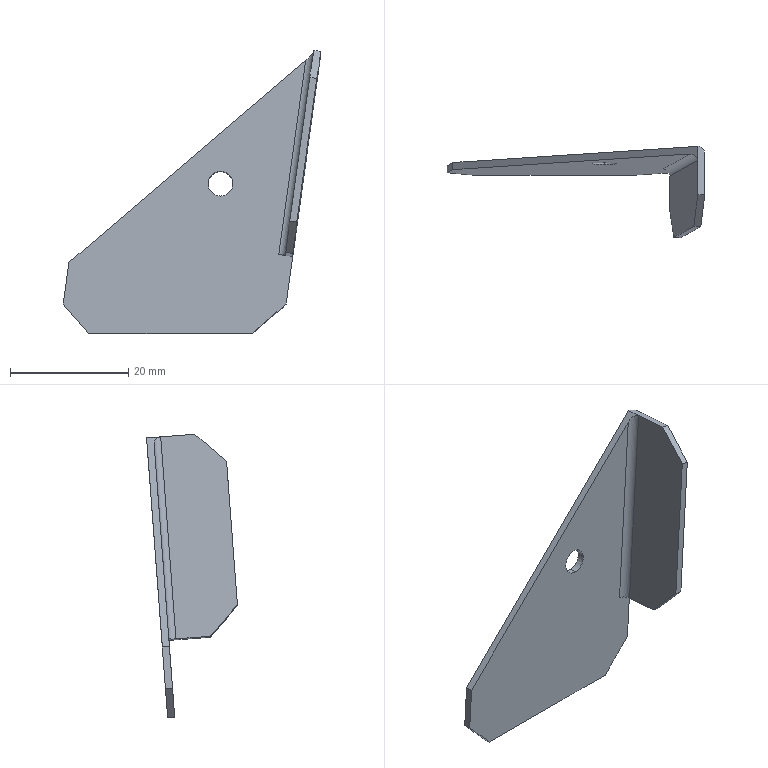Part | SolidWorks | features BaseBody 1 | 1 solid | 18 faces | box 43.581 x 15.38 x 47.955 mm | volume 1791 mm3 | plane 14 | cylinder 4 | commonest cylinder face diameters 2.4 x2 4.2 x2
STEP:
#1=CARTESIAN_POINT('',(232.652,155.946,-588.847));
#2=VERTEX_POINT('',#1);
#3=CARTESIAN_POINT('',(232.652,156.261,-584.659));
#4=VERTEX_POINT('',#3);
#5=CARTESIAN_POINT('',(232.652,156.103,-586.753));
#6=DIRECTION('',(0.,0.9972,-0.07517));
#7=DIRECTION('',(0.,-0.07517,-0.9972));
#8=AXIS2_PLACEMENT_3D('',#5,#6,#7);
#9=CIRCLE('',#8,2.1);
#10=EDGE_CURVE('',#2,#4,#9,.T.);
#11=ORIENTED_EDGE('',*,*,#10,.T.);
#12=CARTESIAN_POINT('',(232.652,155.065,-584.569));
#13=VERTEX_POINT('',#12);
#14=CARTESIAN_POINT('',(232.652,156.261,-584.659));
#15=DIRECTION('',(0.,-0.9972,0.07517));
#16=VECTOR('',#15,1000.);
#17=LINE('',#14,#16);
#18=EDGE_CURVE('',#4,#13,#17,.T.);
#19=ORIENTED_EDGE('',*,*,#18,.T.);
#20=CARTESIAN_POINT('',(232.652,154.749,-588.757));
#21=VERTEX_POINT('',#20);
#22=CARTESIAN_POINT('',(232.652,154.907,-586.663));
#23=DIRECTION('',(0.,-0.9972,0.07517));
#24=DIRECTION('',(0.,-0.07517,-0.9972));
#25=AXIS2_PLACEMENT_3D('',#22,#23,#24);
#26=CIRCLE('',#25,2.1);
#27=EDGE_CURVE('',#13,#21,#26,.T.);
#28=ORIENTED_EDGE('',*,*,#27,.T.);
#29=CARTESIAN_POINT('',(232.652,155.946,-588.847));
#30=DIRECTION('',(0.,-0.9972,0.07517));
#31=VECTOR('',#30,1000.);
#32=LINE('',#29,#31);
#33=EDGE_CURVE('',#2,#21,#32,.T.);
#34=ORIENTED_EDGE('',*,*,#33,.F.);
#35=EDGE_LOOP('',(#11,#19,#28,#34));
#36=FACE_OUTER_BOUND('',#35,.T.);
#37=CARTESIAN_POINT('',(232.652,156.103,-586.753));
#38=DIRECTION('',(0.,-0.9972,0.07517));
#39=DIRECTION('',(0.,-0.07517,-0.9972));
#40=AXIS2_PLACEMENT_3D('',#37,#38,#39);
#41=CYLINDRICAL_SURFACE('',#40,2.1);
#42=ADVANCED_FACE('',(#36),#41,.F.);
#43=CARTESIAN_POINT('',(242.5,154.004,-598.645));
#44=VERTEX_POINT('',#43);
#45=CARTESIAN_POINT('',(243.689,152.795,-598.719));
#46=VERTEX_POINT('',#45);
#47=CARTESIAN_POINT('',(242.5,152.807,-598.555));
#48=DIRECTION('',(-0.1372,-0.07446,-0.9877));
#49=DIRECTION('',(-0.9905,0.,0.1376));
#50=AXIS2_PLACEMENT_3D('',#47,#48,#49);
#51=CIRCLE('',#50,1.2);
#52=EDGE_CURVE('',#44,#46,#51,.T.);
#53=ORIENTED_EDGE('',*,*,#52,.T.);
#54=CARTESIAN_POINT('',(248.438,155.371,-564.537));
#55=VERTEX_POINT('',#54);
#56=CARTESIAN_POINT('',(246.078,154.091,-581.526));
#57=DIRECTION('',(0.1372,0.07446,0.9877));
#58=VECTOR('',#57,1000.);
#59=LINE('',#56,#58);
#60=EDGE_CURVE('',#46,#55,#59,.T.);
#61=ORIENTED_EDGE('',*,*,#60,.T.);
#62=CARTESIAN_POINT('',(248.438,155.384,-564.538));
#63=VERTEX_POINT('',#62);
#64=CARTESIAN_POINT('',(248.438,155.371,-564.537));
#65=CARTESIAN_POINT('',(248.438,155.376,-564.538));
#66=CARTESIAN_POINT('',(248.438,155.38,-564.538));
#67=CARTESIAN_POINT('',(248.438,155.384,-564.538));
#68=(BOUNDED_CURVE()B_SPLINE_CURVE(3,(#64,#65,#66,#67),.UNSPECIFIED.,.F.,.F.)B_SPLINE_CURVE_WITH_KNOTS((4,4),(6.283,6.294),.UNSPECIFIED.)CURVE()GEOMETRIC_REPRESENTATION_ITEM()RATIONAL_B_SPLINE_CURVE((1.,1.,1.,1.))REPRESENTATION_ITEM(''));
#69=EDGE_CURVE('',#55,#63,#68,.T.);
#70=ORIENTED_EDGE('',*,*,#69,.T.);
#71=CARTESIAN_POINT('',(247.063,156.48,-565.801));
#72=VERTEX_POINT('',#71);
#73=CARTESIAN_POINT('',(248.438,155.384,-564.538));
#74=CARTESIAN_POINT('',(248.429,156.078,-564.598));
#75=CARTESIAN_POINT('',(247.862,156.531,-565.119));
#76=CARTESIAN_POINT('',(247.063,156.48,-565.801));
#77=(BOUNDED_CURVE()B_SPLINE_CURVE(3,(#73,#74,#75,#76),.UNSPECIFIED.,.F.,.F.)B_SPLINE_CURVE_WITH_KNOTS((4,4),(3.152,4.712),.UNSPECIFIED.)CURVE()GEOMETRIC_REPRESENTATION_ITEM()RATIONAL_B_SPLINE_CURVE((1.,0.8072,0.8072,1.))REPRESENTATION_ITEM(''));
#78=EDGE_CURVE('',#63,#72,#77,.T.);
#79=ORIENTED_EDGE('',*,*,#78,.T.);
#80=CARTESIAN_POINT('',(244.889,155.3,-581.452));
#81=DIRECTION('',(-0.1372,-0.07446,-0.9877));
#82=VECTOR('',#81,1000.);
#83=LINE('',#80,#82);
#84=EDGE_CURVE('',#72,#44,#83,.T.);
#85=ORIENTED_EDGE('',*,*,#84,.T.);
#86=EDGE_LOOP('',(#53,#61,#70,#79,#85));
#87=FACE_OUTER_BOUND('',#86,.T.);
#88=CARTESIAN_POINT('',(247.277,155.399,-564.168));
#89=DIRECTION('',(-0.1372,-0.07446,-0.9877));
#90=DIRECTION('',(-0.9905,0.,0.1376));
#91=AXIS2_PLACEMENT_3D('',#88,#89,#90);
#92=CYLINDRICAL_SURFACE('',#91,1.2);
#93=ADVANCED_FACE('',(#87),#92,.F.);
#94=ORIENTED_EDGE('',*,*,#60,.F.);
#95=CARTESIAN_POINT('',(243.689,147.011,-598.283));
#96=VERTEX_POINT('',#95);
#97=CARTESIAN_POINT('',(243.689,147.011,-598.283));
#98=DIRECTION('',(0.,0.9972,-0.07517));
#99=VECTOR('',#98,1000.);
#100=LINE('',#97,#99);
#101=EDGE_CURVE('',#96,#46,#100,.T.);
#102=ORIENTED_EDGE('',*,*,#101,.F.);
#103=CARTESIAN_POINT('',(244.375,142.397,-592.968));
#104=VERTEX_POINT('',#103);
#105=CARTESIAN_POINT('',(243.689,147.011,-598.283));
#106=DIRECTION('',(-0.09703,0.6525,-0.7516));
#107=VECTOR('',#106,1000.);
#108=LINE('',#105,#107);
#109=EDGE_CURVE('',#104,#96,#108,.T.);
#110=ORIENTED_EDGE('',*,*,#109,.F.);
#111=CARTESIAN_POINT('',(247.751,144.229,-568.669));
#112=VERTEX_POINT('',#111);
#113=CARTESIAN_POINT('',(247.751,144.229,-568.669));
#114=DIRECTION('',(-0.1372,-0.07446,-0.9877));
#115=VECTOR('',#114,1000.);
#116=LINE('',#113,#115);
#117=EDGE_CURVE('',#112,#104,#116,.T.);
#118=ORIENTED_EDGE('',*,*,#117,.F.);
#119=CARTESIAN_POINT('',(248.438,149.588,-564.101));
#120=VERTEX_POINT('',#119);
#121=CARTESIAN_POINT('',(248.438,149.588,-564.101));
#122=DIRECTION('',(-0.09707,-0.7575,-0.6456));
#123=VECTOR('',#122,1000.);
#124=LINE('',#121,#123);
#125=EDGE_CURVE('',#120,#112,#124,.T.);
#126=ORIENTED_EDGE('',*,*,#125,.F.);
#127=CARTESIAN_POINT('',(248.438,155.371,-564.537));
#128=DIRECTION('',(0.,-0.9972,0.07517));
#129=VECTOR('',#128,1000.);
#130=LINE('',#127,#129);
#131=EDGE_CURVE('',#55,#120,#130,.T.);
#132=ORIENTED_EDGE('',*,*,#131,.F.);
#133=EDGE_LOOP('',(#94,#102,#110,#118,#126,#132));
#134=FACE_OUTER_BOUND('',#133,.T.);
#135=CARTESIAN_POINT('',(243.715,155.371,-598.723));
#136=DIRECTION('',(0.9905,-0.01031,-0.1368));
#137=DIRECTION('',(0.1368,0.,0.9906));
#138=AXIS2_PLACEMENT_3D('',#135,#136,#137);
#139=PLANE('',#138);
#140=ADVANCED_FACE('',(#134),#139,.F.);
#141=CARTESIAN_POINT('',(249.619,156.552,-564.843));
#142=VERTEX_POINT('',#141);
#143=CARTESIAN_POINT('',(249.619,149.572,-564.317));
#144=VERTEX_POINT('',#143);
#145=CARTESIAN_POINT('',(249.619,156.552,-564.843));
#146=DIRECTION('',(0.,-0.9972,0.07517));
#147=VECTOR('',#146,1000.);
#148=LINE('',#145,#147);
#149=EDGE_CURVE('',#142,#144,#148,.T.);
#150=ORIENTED_EDGE('',*,*,#149,.F.);
#151=CARTESIAN_POINT('',(248.438,157.765,-564.718));
#152=VERTEX_POINT('',#151);
#153=CARTESIAN_POINT('',(248.438,157.765,-564.718));
#154=CARTESIAN_POINT('',(249.13,157.755,-564.844));
#155=CARTESIAN_POINT('',(249.619,157.253,-564.896));
#156=CARTESIAN_POINT('',(249.619,156.552,-564.843));
#157=(BOUNDED_CURVE()B_SPLINE_CURVE(3,(#153,#154,#155,#156),.UNSPECIFIED.,.F.,.F.)B_SPLINE_CURVE_WITH_KNOTS((4,4),(4.712,6.283),.UNSPECIFIED.)CURVE()GEOMETRIC_REPRESENTATION_ITEM()RATIONAL_B_SPLINE_CURVE((1.,0.8047,0.8047,1.))REPRESENTATION_ITEM(''));
#158=EDGE_CURVE('',#152,#142,#157,.T.);
#159=ORIENTED_EDGE('',*,*,#158,.F.);
#160=CARTESIAN_POINT('',(248.438,155.384,-564.538));
#161=DIRECTION('',(0.,0.9972,-0.07517));
#162=VECTOR('',#161,1000.);
#163=LINE('',#160,#162);
#164=EDGE_CURVE('',#63,#152,#163,.T.);
#165=ORIENTED_EDGE('',*,*,#164,.F.);
#166=ORIENTED_EDGE('',*,*,#69,.F.);
#167=ORIENTED_EDGE('',*,*,#131,.T.);
#168=CARTESIAN_POINT('',(248.429,149.588,-564.1));
#169=DIRECTION('',(-0.9837,0.01354,0.1796));
#170=VECTOR('',#169,1000.);
#171=LINE('',#168,#170);
#172=EDGE_CURVE('',#144,#120,#171,.T.);
#173=ORIENTED_EDGE('',*,*,#172,.F.);
#174=EDGE_LOOP('',(#150,#159,#165,#166,#167,#173));
#175=FACE_OUTER_BOUND('',#174,.T.);
#176=CARTESIAN_POINT('',(248.32,157.814,-564.7));
#177=DIRECTION('',(-0.1801,-0.07394,-0.9809));
#178=DIRECTION('',(0.9836,0.,-0.1806));
#179=AXIS2_PLACEMENT_3D('',#176,#177,#178);
#180=PLANE('',#179);
#181=ADVANCED_FACE('',(#175),#180,.F.);
#182=ORIENTED_EDGE('',*,*,#101,.T.);
#183=ORIENTED_EDGE('',*,*,#52,.F.);
#184=CARTESIAN_POINT('',(244.878,153.979,-598.973));
#185=VERTEX_POINT('',#184);
#186=CARTESIAN_POINT('',(244.878,153.979,-598.973));
#187=DIRECTION('',(-0.9905,0.01031,0.1368));
#188=VECTOR('',#187,1000.);
#189=LINE('',#186,#188);
#190=EDGE_CURVE('',#185,#44,#189,.T.);
#191=ORIENTED_EDGE('',*,*,#190,.F.);
#192=CARTESIAN_POINT('',(244.878,146.999,-598.447));
#193=VERTEX_POINT('',#192);
#194=CARTESIAN_POINT('',(244.878,146.999,-598.447));
#195=DIRECTION('',(0.,0.9972,-0.07517));
#196=VECTOR('',#195,1000.);
#197=LINE('',#194,#196);
#198=EDGE_CURVE('',#193,#185,#197,.T.);
#199=ORIENTED_EDGE('',*,*,#198,.F.);
#200=CARTESIAN_POINT('',(243.689,147.011,-598.283));
#201=DIRECTION('',(0.9905,-0.01031,-0.1368));
#202=VECTOR('',#201,1000.);
#203=LINE('',#200,#202);
#204=EDGE_CURVE('',#96,#193,#203,.T.);
#205=ORIENTED_EDGE('',*,*,#204,.F.);
#206=EDGE_LOOP('',(#182,#183,#191,#199,#205));
#207=FACE_OUTER_BOUND('',#206,.T.);
#208=CARTESIAN_POINT('',(244.891,154.046,-598.98));
#209=DIRECTION('',(0.1372,0.07446,0.9877));
#210=DIRECTION('',(-0.9905,0.,0.1376));
#211=AXIS2_PLACEMENT_3D('',#208,#209,#210);
#212=PLANE('',#211);
#213=ADVANCED_FACE('',(#207),#212,.F.);
#214=ORIENTED_EDGE('',*,*,#109,.T.);
#215=ORIENTED_EDGE('',*,*,#204,.T.);
#216=CARTESIAN_POINT('',(245.564,142.385,-593.133));
#217=VERTEX_POINT('',#216);
#218=CARTESIAN_POINT('',(245.221,144.692,-595.79));
#219=DIRECTION('',(0.09703,-0.6525,0.7516));
#220=VECTOR('',#219,1000.);
#221=LINE('',#218,#220);
#222=EDGE_CURVE('',#193,#217,#221,.T.);
#223=ORIENTED_EDGE('',*,*,#222,.T.);
#224=CARTESIAN_POINT('',(244.97,142.391,-593.05));
#225=DIRECTION('',(-0.9905,0.01031,0.1368));
#226=VECTOR('',#225,1000.);
#227=LINE('',#224,#226);
#228=EDGE_CURVE('',#217,#104,#227,.T.);
#229=ORIENTED_EDGE('',*,*,#228,.T.);
#230=EDGE_LOOP('',(#214,#215,#223,#229));
#231=FACE_OUTER_BOUND('',#230,.T.);
#232=CARTESIAN_POINT('',(243.689,147.011,-598.283));
#233=DIRECTION('',(-0.09703,-0.7578,-0.6453));
#234=DIRECTION('',(0.9905,-0.01031,-0.1368));
#235=AXIS2_PLACEMENT_3D('',#232,#233,#234);
#236=PLANE('',#235);
#237=ADVANCED_FACE('',(#231),#236,.T.);
#238=CARTESIAN_POINT('',(248.932,144.213,-568.884));
#239=VERTEX_POINT('',#238);
#240=CARTESIAN_POINT('',(245.564,142.385,-593.133));
#241=DIRECTION('',(0.1372,0.07446,0.9877));
#242=VECTOR('',#241,1000.);
#243=LINE('',#240,#242);
#244=EDGE_CURVE('',#217,#239,#243,.T.);
#245=ORIENTED_EDGE('',*,*,#244,.T.);
#246=CARTESIAN_POINT('',(248.932,144.213,-568.884));
#247=DIRECTION('',(-0.9837,0.01354,0.1796));
#248=VECTOR('',#247,1000.);
#249=LINE('',#246,#248);
#250=EDGE_CURVE('',#239,#112,#249,.T.);
#251=ORIENTED_EDGE('',*,*,#250,.T.);
#252=ORIENTED_EDGE('',*,*,#117,.T.);
#253=ORIENTED_EDGE('',*,*,#228,.F.);
#254=EDGE_LOOP('',(#245,#251,#252,#253));
#255=FACE_OUTER_BOUND('',#254,.T.);
#256=CARTESIAN_POINT('',(248.96,142.374,-593.279));
#257=DIRECTION('',(0.,-0.9972,0.07517));
#258=DIRECTION('',(0.,0.07517,0.9972));
#259=AXIS2_PLACEMENT_3D('',#256,#257,#258);
#260=PLANE('',#259);
#261=ADVANCED_FACE('',(#255),#260,.T.);
#262=ORIENTED_EDGE('',*,*,#125,.T.);
#263=ORIENTED_EDGE('',*,*,#250,.F.);
#264=CARTESIAN_POINT('',(248.932,144.213,-568.884));
#265=DIRECTION('',(0.09707,0.7575,0.6456));
#266=VECTOR('',#265,1000.);
#267=LINE('',#264,#266);
#268=EDGE_CURVE('',#239,#144,#267,.T.);
#269=ORIENTED_EDGE('',*,*,#268,.T.);
#270=ORIENTED_EDGE('',*,*,#172,.T.);
#271=EDGE_LOOP('',(#262,#263,#269,#270));
#272=FACE_OUTER_BOUND('',#271,.T.);
#273=CARTESIAN_POINT('',(247.529,144.232,-568.628));
#274=DIRECTION('',(0.1273,-0.6528,0.7467));
#275=DIRECTION('',(0.9837,-0.01354,-0.1796));
#276=AXIS2_PLACEMENT_3D('',#273,#274,#275);
#277=PLANE('',#276);
#278=ADVANCED_FACE('',(#272),#277,.T.);
#279=CARTESIAN_POINT('',(232.652,154.907,-586.663));
#280=DIRECTION('',(0.,-0.9972,0.07517));
#281=DIRECTION('',(0.,-0.07517,-0.9972));
#282=AXIS2_PLACEMENT_3D('',#279,#280,#281);
#283=CIRCLE('',#282,2.1);
#284=EDGE_CURVE('',#21,#13,#283,.T.);
#285=ORIENTED_EDGE('',*,*,#284,.F.);
#286=ORIENTED_EDGE('',*,*,#27,.F.);
#287=EDGE_LOOP('',(#285,#286));
#288=FACE_BOUND('',#287,.T.);
#289=CARTESIAN_POINT('',(206.038,153.372,-607.027));
#290=VERTEX_POINT('',#289);
#291=CARTESIAN_POINT('',(207.014,153.901,-600.));
#292=VERTEX_POINT('',#291);
#293=CARTESIAN_POINT('',(206.038,153.372,-607.027));
#294=DIRECTION('',(0.1372,0.07446,0.9877));
#295=VECTOR('',#294,1000.);
#296=LINE('',#293,#295);
#297=EDGE_CURVE('',#290,#292,#296,.T.);
#298=ORIENTED_EDGE('',*,*,#297,.F.);
#299=CARTESIAN_POINT('',(210.352,152.999,-611.966));
#300=VERTEX_POINT('',#299);
#301=CARTESIAN_POINT('',(210.352,152.999,-611.966));
#302=DIRECTION('',(-0.6568,0.05669,0.7519));
#303=VECTOR('',#302,1000.);
#304=LINE('',#301,#303);
#305=EDGE_CURVE('',#300,#290,#304,.T.);
#306=ORIENTED_EDGE('',*,*,#305,.F.);
#307=CARTESIAN_POINT('',(238.073,152.999,-611.966));
#308=VERTEX_POINT('',#307);
#309=CARTESIAN_POINT('',(226.55,152.999,-611.966));
#310=DIRECTION('',(-1.,0.,0.));
#311=VECTOR('',#310,1000.);
#312=LINE('',#309,#311);
#313=EDGE_CURVE('',#308,#300,#312,.T.);
#314=ORIENTED_EDGE('',*,*,#313,.F.);
#315=CARTESIAN_POINT('',(243.759,153.372,-607.027));
#316=VERTEX_POINT('',#315);
#317=CARTESIAN_POINT('',(243.759,153.372,-607.027));
#318=DIRECTION('',(-0.7541,-0.04937,-0.6549));
#319=VECTOR('',#318,1000.);
#320=LINE('',#317,#319);
#321=EDGE_CURVE('',#316,#308,#320,.T.);
#322=ORIENTED_EDGE('',*,*,#321,.F.);
#323=CARTESIAN_POINT('',(249.619,156.552,-564.843));
#324=DIRECTION('',(-0.1372,-0.07446,-0.9877));
#325=VECTOR('',#324,1000.);
#326=LINE('',#323,#325);
#327=EDGE_CURVE('',#185,#316,#326,.T.);
#328=ORIENTED_EDGE('',*,*,#327,.F.);
#329=ORIENTED_EDGE('',*,*,#190,.T.);
#330=ORIENTED_EDGE('',*,*,#84,.F.);
#331=CARTESIAN_POINT('',(207.014,153.901,-600.));
#332=DIRECTION('',(0.7596,0.0489,0.6486));
#333=VECTOR('',#332,1000.);
#334=LINE('',#331,#333);
#335=EDGE_CURVE('',#292,#72,#334,.T.);
#336=ORIENTED_EDGE('',*,*,#335,.F.);
#337=EDGE_LOOP('',(#298,#306,#314,#322,#328,#329,#330,#336));
#338=FACE_OUTER_BOUND('',#337,.T.);
#339=CARTESIAN_POINT('',(247.309,156.5,-565.524));
#340=DIRECTION('',(0.,0.9972,-0.07517));
#341=DIRECTION('',(0.,-0.07517,-0.9972));
#342=AXIS2_PLACEMENT_3D('',#339,#340,#341);
#343=PLANE('',#342);
#344=ADVANCED_FACE('',(#288,#338),#343,.F.);
#345=CARTESIAN_POINT('',(207.014,155.098,-600.09));
#346=VERTEX_POINT('',#345);
#347=CARTESIAN_POINT('',(207.014,153.901,-600.));
#348=DIRECTION('',(-0.000000001,0.9972,-0.07517));
#349=VECTOR('',#348,1000.);
#350=LINE('',#347,#349);
#351=EDGE_CURVE('',#292,#346,#350,.T.);
#352=ORIENTED_EDGE('',*,*,#351,.F.);
#353=ORIENTED_EDGE('',*,*,#335,.T.);
#354=ORIENTED_EDGE('',*,*,#78,.F.);
#355=ORIENTED_EDGE('',*,*,#164,.T.);
#356=CARTESIAN_POINT('',(207.014,155.098,-600.09));
#357=DIRECTION('',(0.7596,0.0489,0.6486));
#358=VECTOR('',#357,1000.);
#359=LINE('',#356,#358);
#360=EDGE_CURVE('',#346,#152,#359,.T.);
#361=ORIENTED_EDGE('',*,*,#360,.F.);
#362=EDGE_LOOP('',(#352,#353,#354,#355,#361));
#363=FACE_OUTER_BOUND('',#362,.T.);
#364=CARTESIAN_POINT('',(206.866,157.788,-600.42));
#365=DIRECTION('',(0.6504,-0.0571,-0.7574));
#366=DIRECTION('',(0.7586,0.,0.6515));
#367=AXIS2_PLACEMENT_3D('',#364,#365,#366);
#368=PLANE('',#367);
#369=ADVANCED_FACE('',(#363),#368,.F.);
#370=ORIENTED_EDGE('',*,*,#222,.F.);
#371=ORIENTED_EDGE('',*,*,#198,.T.);
#372=CARTESIAN_POINT('',(249.619,156.552,-564.843));
#373=DIRECTION('',(-0.1372,-0.07446,-0.9877));
#374=VECTOR('',#373,1000.);
#375=LINE('',#372,#374);
#376=EDGE_CURVE('',#142,#185,#375,.T.);
#377=ORIENTED_EDGE('',*,*,#376,.F.);
#378=ORIENTED_EDGE('',*,*,#149,.T.);
#379=ORIENTED_EDGE('',*,*,#268,.F.);
#380=ORIENTED_EDGE('',*,*,#244,.F.);
#381=EDGE_LOOP('',(#370,#371,#377,#378,#379,#380));
#382=FACE_OUTER_BOUND('',#381,.T.);
#383=CARTESIAN_POINT('',(249.69,156.552,-564.327));
#384=DIRECTION('',(-0.9905,0.01031,0.1368));
#385=DIRECTION('',(-0.1368,0.,-0.9906));
#386=AXIS2_PLACEMENT_3D('',#383,#384,#385);
#387=PLANE('',#386);
#388=ADVANCED_FACE('',(#382),#387,.F.);
#389=ORIENTED_EDGE('',*,*,#158,.T.);
#390=ORIENTED_EDGE('',*,*,#376,.T.);
#391=ORIENTED_EDGE('',*,*,#327,.T.);
#392=CARTESIAN_POINT('',(242.381,154.478,-608.314));
#393=VERTEX_POINT('',#392);
#394=CARTESIAN_POINT('',(242.381,154.478,-608.314));
#395=CARTESIAN_POINT('',(243.188,154.531,-607.613));
#396=CARTESIAN_POINT('',(243.759,154.073,-607.08));
#397=CARTESIAN_POINT('',(243.759,153.372,-607.027));
#398=(BOUNDED_CURVE()B_SPLINE_CURVE(3,(#394,#395,#396,#397),.UNSPECIFIED.,.F.,.F.)B_SPLINE_CURVE_WITH_KNOTS((4,4),(1.571,3.142),.UNSPECIFIED.)CURVE()GEOMETRIC_REPRESENTATION_ITEM()RATIONAL_B_SPLINE_CURVE((1.,0.8047,0.8047,1.))REPRESENTATION_ITEM(''));
#399=EDGE_CURVE('',#393,#316,#398,.T.);
#400=ORIENTED_EDGE('',*,*,#399,.F.);
#401=CARTESIAN_POINT('',(245.409,156.121,-586.516));
#402=DIRECTION('',(-0.1372,-0.07446,-0.9877));
#403=VECTOR('',#402,1000.);
#404=LINE('',#401,#403);
#405=EDGE_CURVE('',#152,#393,#404,.T.);
#406=ORIENTED_EDGE('',*,*,#405,.F.);
#407=EDGE_LOOP('',(#389,#390,#391,#400,#406));
#408=FACE_OUTER_BOUND('',#407,.T.);
#409=CARTESIAN_POINT('',(248.474,156.588,-564.366));
#410=DIRECTION('',(-0.1372,-0.07446,-0.9877));
#411=DIRECTION('',(-0.9905,0.,0.1376));
#412=AXIS2_PLACEMENT_3D('',#409,#410,#411);
#413=CYLINDRICAL_SURFACE('',#412,1.2);
#414=ADVANCED_FACE('',(#408),#413,.T.);
#415=ORIENTED_EDGE('',*,*,#18,.F.);
#416=CARTESIAN_POINT('',(232.652,156.103,-586.753));
#417=DIRECTION('',(0.,0.9972,-0.07517));
#418=DIRECTION('',(0.,-0.07517,-0.9972));
#419=AXIS2_PLACEMENT_3D('',#416,#417,#418);
#420=CIRCLE('',#419,2.1);
#421=EDGE_CURVE('',#4,#2,#420,.T.);
#422=ORIENTED_EDGE('',*,*,#421,.T.);
#423=ORIENTED_EDGE('',*,*,#33,.T.);
#424=ORIENTED_EDGE('',*,*,#284,.T.);
#425=EDGE_LOOP('',(#415,#422,#423,#424));
#426=FACE_OUTER_BOUND('',#425,.T.);
#427=CARTESIAN_POINT('',(232.652,156.103,-586.753));
#428=DIRECTION('',(0.,-0.9972,0.07517));
#429=DIRECTION('',(0.,-0.07517,-0.9972));
#430=AXIS2_PLACEMENT_3D('',#427,#428,#429);
#431=CYLINDRICAL_SURFACE('',#430,2.1);
#432=ADVANCED_FACE('',(#426),#431,.F.);
#433=ORIENTED_EDGE('',*,*,#351,.T.);
#434=CARTESIAN_POINT('',(206.038,154.568,-607.118));
#435=VERTEX_POINT('',#434);
#436=CARTESIAN_POINT('',(206.038,154.568,-607.118));
#437=DIRECTION('',(0.1372,0.07446,0.9877));
#438=VECTOR('',#437,1000.);
#439=LINE('',#436,#438);
#440=EDGE_CURVE('',#435,#346,#439,.T.);
#441=ORIENTED_EDGE('',*,*,#440,.F.);
#442=CARTESIAN_POINT('',(206.038,153.372,-607.027));
#443=DIRECTION('',(0.,0.9972,-0.07517));
#444=VECTOR('',#443,1000.);
#445=LINE('',#442,#444);
#446=EDGE_CURVE('',#290,#435,#445,.T.);
#447=ORIENTED_EDGE('',*,*,#446,.F.);
#448=ORIENTED_EDGE('',*,*,#297,.T.);
#449=EDGE_LOOP('',(#433,#441,#447,#448));
#450=FACE_OUTER_BOUND('',#449,.T.);
#451=CARTESIAN_POINT('',(206.037,155.108,-607.161));
#452=DIRECTION('',(0.9905,-0.01031,-0.1368));
#453=DIRECTION('',(0.1368,0.,0.9906));
#454=AXIS2_PLACEMENT_3D('',#451,#452,#453);
#455=PLANE('',#454);
#456=ADVANCED_FACE('',(#450),#455,.F.);
#457=ORIENTED_EDGE('',*,*,#446,.T.);
#458=CARTESIAN_POINT('',(210.352,154.196,-612.056));
#459=VERTEX_POINT('',#458);
#460=CARTESIAN_POINT('',(210.352,154.196,-612.056));
#461=DIRECTION('',(-0.6568,0.05669,0.7519));
#462=VECTOR('',#461,1000.);
#463=LINE('',#460,#462);
#464=EDGE_CURVE('',#459,#435,#463,.T.);
#465=ORIENTED_EDGE('',*,*,#464,.F.);
#466=CARTESIAN_POINT('',(210.352,152.999,-611.966));
#467=DIRECTION('',(0.,0.9972,-0.07517));
#468=VECTOR('',#467,1000.);
#469=LINE('',#466,#468);
#470=EDGE_CURVE('',#300,#459,#469,.T.);
#471=ORIENTED_EDGE('',*,*,#470,.F.);
#472=ORIENTED_EDGE('',*,*,#305,.T.);
#473=EDGE_LOOP('',(#457,#465,#471,#472));
#474=FACE_OUTER_BOUND('',#473,.T.);
#475=CARTESIAN_POINT('',(210.364,154.578,-612.099));
#476=DIRECTION('',(0.7541,0.04937,0.6549));
#477=DIRECTION('',(-0.6557,0.,0.755));
#478=AXIS2_PLACEMENT_3D('',#475,#476,#477);
#479=PLANE('',#478);
#480=ADVANCED_FACE('',(#474),#479,.F.);
#481=ORIENTED_EDGE('',*,*,#470,.T.);
#482=CARTESIAN_POINT('',(238.073,154.196,-612.056));
#483=VERTEX_POINT('',#482);
#484=CARTESIAN_POINT('',(224.212,154.196,-612.056));
#485=DIRECTION('',(-1.,0.,0.));
#486=VECTOR('',#485,1000.);
#487=LINE('',#484,#486);
#488=EDGE_CURVE('',#483,#459,#487,.T.);
#489=ORIENTED_EDGE('',*,*,#488,.F.);
#490=CARTESIAN_POINT('',(238.073,153.598,-612.011));
#491=DIRECTION('',(0.,0.9972,-0.07517));
#492=VECTOR('',#491,1000.);
#493=LINE('',#490,#492);
#494=EDGE_CURVE('',#308,#483,#493,.T.);
#495=ORIENTED_EDGE('',*,*,#494,.F.);
#496=ORIENTED_EDGE('',*,*,#313,.T.);
#497=EDGE_LOOP('',(#481,#489,#495,#496));
#498=FACE_OUTER_BOUND('',#497,.T.);
#499=CARTESIAN_POINT('',(238.073,152.999,-611.966));
#500=DIRECTION('',(0.,0.07517,0.9972));
#501=DIRECTION('',(0.,0.9972,-0.07517));
#502=AXIS2_PLACEMENT_3D('',#499,#500,#501);
#503=PLANE('',#502);
#504=ADVANCED_FACE('',(#498),#503,.F.);
#505=ORIENTED_EDGE('',*,*,#494,.T.);
#506=CARTESIAN_POINT('',(242.381,154.478,-608.314));
#507=DIRECTION('',(-0.7541,-0.04937,-0.6549));
#508=VECTOR('',#507,1000.);
#509=LINE('',#506,#508);
#510=EDGE_CURVE('',#393,#483,#509,.T.);
#511=ORIENTED_EDGE('',*,*,#510,.F.);
#512=ORIENTED_EDGE('',*,*,#399,.T.);
#513=ORIENTED_EDGE('',*,*,#321,.T.);
#514=EDGE_LOOP('',(#505,#511,#512,#513));
#515=FACE_OUTER_BOUND('',#514,.T.);
#516=CARTESIAN_POINT('',(243.835,154.49,-607.045));
#517=DIRECTION('',(-0.6568,0.05669,0.7519));
#518=DIRECTION('',(-0.7531,0.,-0.6579));
#519=AXIS2_PLACEMENT_3D('',#516,#517,#518);
#520=PLANE('',#519);
#521=ADVANCED_FACE('',(#515),#520,.F.);
#522=ORIENTED_EDGE('',*,*,#10,.F.);
#523=ORIENTED_EDGE('',*,*,#421,.F.);
#524=EDGE_LOOP('',(#522,#523));
#525=FACE_BOUND('',#524,.T.);
#526=ORIENTED_EDGE('',*,*,#360,.T.);
#527=ORIENTED_EDGE('',*,*,#405,.T.);
#528=ORIENTED_EDGE('',*,*,#510,.T.);
#529=ORIENTED_EDGE('',*,*,#488,.T.);
#530=ORIENTED_EDGE('',*,*,#464,.T.);
#531=ORIENTED_EDGE('',*,*,#440,.T.);
#532=EDGE_LOOP('',(#526,#527,#528,#529,#530,#531));
#533=FACE_OUTER_BOUND('',#532,.T.);
#534=CARTESIAN_POINT('',(248.692,157.786,-564.434));
#535=DIRECTION('',(0.,0.9972,-0.07517));
#536=DIRECTION('',(0.,-0.07517,-0.9972));
#537=AXIS2_PLACEMENT_3D('',#534,#535,#536);
#538=PLANE('',#537);
#539=ADVANCED_FACE('',(#525,#533),#538,.T.);
#540=CLOSED_SHELL('',(#42,#93,#140,#181,#213,#237,#261,#278,#344,#369,#388,#414,#432,#456,#480,#504,#521,#539));
#541=MANIFOLD_SOLID_BREP('',#540);
#542=CARTESIAN_POINT('',(0.,0.,0.));
#543=DIRECTION('',(0.,0.,1.));
#544=DIRECTION('',(1.,0.,0.));
#545=AXIS2_PLACEMENT_3D('',#542,#543,#544);
#546=(LENGTH_UNIT()NAMED_UNIT(*)SI_UNIT(.MILLI.,.METRE.));
#547=UNCERTAINTY_MEASURE_WITH_UNIT(LENGTH_MEASURE(0.00001),#546,'','');
#548=(NAMED_UNIT(*)PLANE_ANGLE_UNIT()SI_UNIT($,.RADIAN.));
#549=(NAMED_UNIT(*)SI_UNIT($,.STERADIAN.)SOLID_ANGLE_UNIT());
#550=(GEOMETRIC_REPRESENTATION_CONTEXT(3)GLOBAL_UNCERTAINTY_ASSIGNED_CONTEXT((#547))GLOBAL_UNIT_ASSIGNED_CONTEXT((#546,#548,#549))REPRESENTATION_CONTEXT('',''));
#551=ADVANCED_BREP_SHAPE_REPRESENTATION('',(#541,#545),#550);